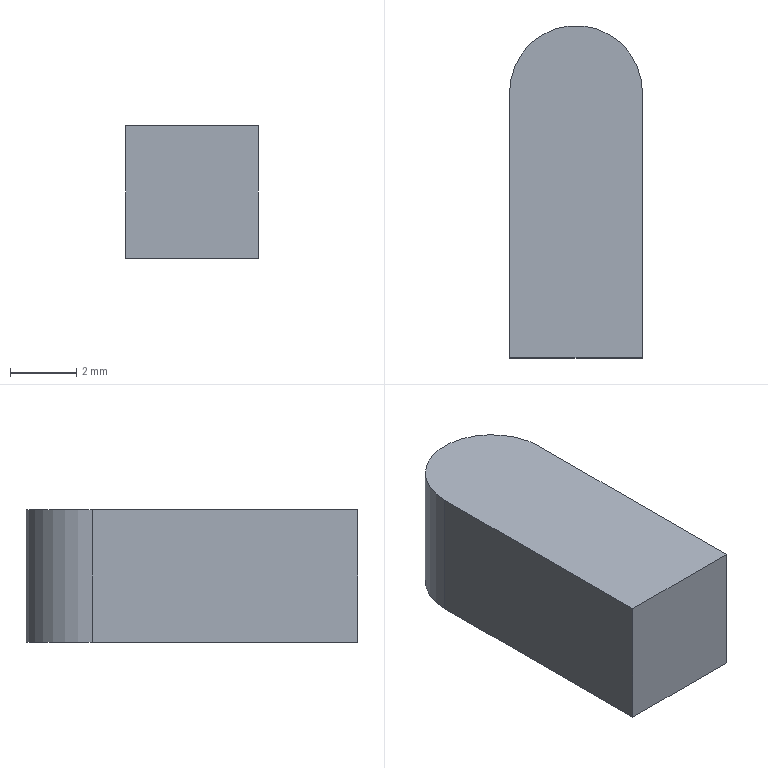Part | NX | features DATUM_CSYS 2, EXTRUDE 1, FACE_BLEND 1, SKETCH 1 | 1 solid | 6 faces | box 4 x 10 x 4 mm | volume 153.133 mm3 | plane 5 | cylinder 1 | commonest cylinder face diameters 4 x1
STEP:
#1=CARTESIAN_POINT('',(2.,8.,0.));
#2=VERTEX_POINT('',#1);
#3=CARTESIAN_POINT('',(2.,8.,4.));
#4=VERTEX_POINT('',#3);
#5=CARTESIAN_POINT('',(2.,8.,4.));
#6=DIRECTION('',(0.,0.,1.));
#7=VECTOR('',#6,1000.);
#8=LINE('',#5,#7);
#9=EDGE_CURVE('',#2,#4,#8,.T.);
#10=ORIENTED_EDGE('',*,*,#9,.F.);
#11=CARTESIAN_POINT('',(-2.,8.,0.));
#12=VERTEX_POINT('',#11);
#13=CARTESIAN_POINT('',(0.,8.,0.));
#14=DIRECTION('',(0.,0.,1.));
#15=DIRECTION('',(1.,0.,0.));
#16=AXIS2_PLACEMENT_3D('',#13,#14,#15);
#17=CIRCLE('',#16,2.);
#18=EDGE_CURVE('',#12,#2,#17,.F.);
#19=ORIENTED_EDGE('',*,*,#18,.F.);
#20=CARTESIAN_POINT('',(-2.,8.,4.));
#21=VERTEX_POINT('',#20);
#22=CARTESIAN_POINT('',(-2.,8.,4.));
#23=DIRECTION('',(0.,0.,1.));
#24=VECTOR('',#23,1000.);
#25=LINE('',#22,#24);
#26=EDGE_CURVE('',#21,#12,#25,.F.);
#27=ORIENTED_EDGE('',*,*,#26,.F.);
#28=CARTESIAN_POINT('',(0.,8.,4.));
#29=DIRECTION('',(0.,0.,1.));
#30=DIRECTION('',(1.,0.,0.));
#31=AXIS2_PLACEMENT_3D('',#28,#29,#30);
#32=CIRCLE('',#31,2.);
#33=EDGE_CURVE('',#4,#21,#32,.T.);
#34=ORIENTED_EDGE('',*,*,#33,.F.);
#35=EDGE_LOOP('',(#10,#19,#27,#34));
#36=FACE_BOUND('',#35,.T.);
#37=CARTESIAN_POINT('',(0.,8.,0.));
#38=DIRECTION('',(0.,0.,1.));
#39=DIRECTION('',(1.,0.,0.));
#40=AXIS2_PLACEMENT_3D('',#37,#38,#39);
#41=CYLINDRICAL_SURFACE('',#40,2.);
#42=ADVANCED_FACE('',(#36),#41,.T.);
#43=CARTESIAN_POINT('',(-2.,0.,4.));
#44=VERTEX_POINT('',#43);
#45=CARTESIAN_POINT('',(-2.,10.,4.));
#46=DIRECTION('',(0.,-1.,0.));
#47=VECTOR('',#46,1000.);
#48=LINE('',#45,#47);
#49=EDGE_CURVE('',#21,#44,#48,.T.);
#50=ORIENTED_EDGE('',*,*,#49,.F.);
#51=ORIENTED_EDGE('',*,*,#26,.T.);
#52=CARTESIAN_POINT('',(-2.,0.,0.));
#53=VERTEX_POINT('',#52);
#54=CARTESIAN_POINT('',(-2.,10.,0.));
#55=DIRECTION('',(0.,-1.,0.));
#56=VECTOR('',#55,1000.);
#57=LINE('',#54,#56);
#58=EDGE_CURVE('',#12,#53,#57,.T.);
#59=ORIENTED_EDGE('',*,*,#58,.T.);
#60=CARTESIAN_POINT('',(-2.,0.,4.));
#61=DIRECTION('',(0.,0.,-1.));
#62=VECTOR('',#61,1000.);
#63=LINE('',#60,#62);
#64=EDGE_CURVE('',#44,#53,#63,.T.);
#65=ORIENTED_EDGE('',*,*,#64,.F.);
#66=EDGE_LOOP('',(#50,#51,#59,#65));
#67=FACE_BOUND('',#66,.T.);
#68=CARTESIAN_POINT('',(-2.,10.,4.));
#69=DIRECTION('',(1.,0.,0.));
#70=DIRECTION('',(0.,1.,0.));
#71=AXIS2_PLACEMENT_3D('',#68,#69,#70);
#72=PLANE('',#71);
#73=ADVANCED_FACE('',(#67),#72,.F.);
#74=CARTESIAN_POINT('',(2.,0.,0.));
#75=VERTEX_POINT('',#74);
#76=CARTESIAN_POINT('',(-2.,0.,0.));
#77=DIRECTION('',(1.,0.,0.));
#78=VECTOR('',#77,1000.);
#79=LINE('',#76,#78);
#80=EDGE_CURVE('',#53,#75,#79,.T.);
#81=ORIENTED_EDGE('',*,*,#80,.T.);
#82=CARTESIAN_POINT('',(2.,0.,4.));
#83=VERTEX_POINT('',#82);
#84=CARTESIAN_POINT('',(2.,0.,4.));
#85=DIRECTION('',(0.,0.,-1.));
#86=VECTOR('',#85,1000.);
#87=LINE('',#84,#86);
#88=EDGE_CURVE('',#83,#75,#87,.T.);
#89=ORIENTED_EDGE('',*,*,#88,.F.);
#90=CARTESIAN_POINT('',(-2.,0.,4.));
#91=DIRECTION('',(1.,0.,0.));
#92=VECTOR('',#91,1000.);
#93=LINE('',#90,#92);
#94=EDGE_CURVE('',#44,#83,#93,.T.);
#95=ORIENTED_EDGE('',*,*,#94,.F.);
#96=ORIENTED_EDGE('',*,*,#64,.T.);
#97=EDGE_LOOP('',(#81,#89,#95,#96));
#98=FACE_BOUND('',#97,.T.);
#99=CARTESIAN_POINT('',(-2.,0.,4.));
#100=DIRECTION('',(0.,1.,0.));
#101=DIRECTION('',(0.,0.,1.));
#102=AXIS2_PLACEMENT_3D('',#99,#100,#101);
#103=PLANE('',#102);
#104=ADVANCED_FACE('',(#98),#103,.F.);
#105=CARTESIAN_POINT('',(2.,0.,0.));
#106=DIRECTION('',(0.,1.,0.));
#107=VECTOR('',#106,1000.);
#108=LINE('',#105,#107);
#109=EDGE_CURVE('',#75,#2,#108,.T.);
#110=ORIENTED_EDGE('',*,*,#109,.T.);
#111=ORIENTED_EDGE('',*,*,#9,.T.);
#112=CARTESIAN_POINT('',(2.,0.,4.));
#113=DIRECTION('',(0.,1.,0.));
#114=VECTOR('',#113,1000.);
#115=LINE('',#112,#114);
#116=EDGE_CURVE('',#83,#4,#115,.T.);
#117=ORIENTED_EDGE('',*,*,#116,.F.);
#118=ORIENTED_EDGE('',*,*,#88,.T.);
#119=EDGE_LOOP('',(#110,#111,#117,#118));
#120=FACE_BOUND('',#119,.T.);
#121=CARTESIAN_POINT('',(2.,0.,4.));
#122=DIRECTION('',(-1.,0.,0.));
#123=DIRECTION('',(0.,-1.,0.));
#124=AXIS2_PLACEMENT_3D('',#121,#122,#123);
#125=PLANE('',#124);
#126=ADVANCED_FACE('',(#120),#125,.F.);
#127=ORIENTED_EDGE('',*,*,#116,.T.);
#128=ORIENTED_EDGE('',*,*,#33,.T.);
#129=ORIENTED_EDGE('',*,*,#49,.T.);
#130=ORIENTED_EDGE('',*,*,#94,.T.);
#131=EDGE_LOOP('',(#127,#128,#129,#130));
#132=FACE_BOUND('',#131,.T.);
#133=CARTESIAN_POINT('',(0.,0.,4.));
#134=DIRECTION('',(0.,0.,1.));
#135=DIRECTION('',(1.,0.,0.));
#136=AXIS2_PLACEMENT_3D('',#133,#134,#135);
#137=PLANE('',#136);
#138=ADVANCED_FACE('',(#132),#137,.T.);
#139=ORIENTED_EDGE('',*,*,#58,.F.);
#140=ORIENTED_EDGE('',*,*,#18,.T.);
#141=ORIENTED_EDGE('',*,*,#109,.F.);
#142=ORIENTED_EDGE('',*,*,#80,.F.);
#143=EDGE_LOOP('',(#139,#140,#141,#142));
#144=FACE_BOUND('',#143,.T.);
#145=CARTESIAN_POINT('',(0.,0.,0.));
#146=DIRECTION('',(0.,0.,1.));
#147=DIRECTION('',(1.,0.,0.));
#148=AXIS2_PLACEMENT_3D('',#145,#146,#147);
#149=PLANE('',#148);
#150=ADVANCED_FACE('',(#144),#149,.F.);
#151=CLOSED_SHELL('',(#42,#73,#104,#126,#138,#150));
#152=MANIFOLD_SOLID_BREP('',#151);
#153=(LENGTH_UNIT()NAMED_UNIT(*)SI_UNIT(.MILLI.,.METRE.));
#154=UNCERTAINTY_MEASURE_WITH_UNIT(LENGTH_MEASURE(0.00001),#153,'','');
#155=(NAMED_UNIT(*)PLANE_ANGLE_UNIT()SI_UNIT($,.RADIAN.));
#156=(NAMED_UNIT(*)SI_UNIT($,.STERADIAN.)SOLID_ANGLE_UNIT());
#157=(GEOMETRIC_REPRESENTATION_CONTEXT(3)GLOBAL_UNCERTAINTY_ASSIGNED_CONTEXT((#154))GLOBAL_UNIT_ASSIGNED_CONTEXT((#153,#155,#156))REPRESENTATION_CONTEXT('',''));
#158=ADVANCED_BREP_SHAPE_REPRESENTATION('',(#152),#157);